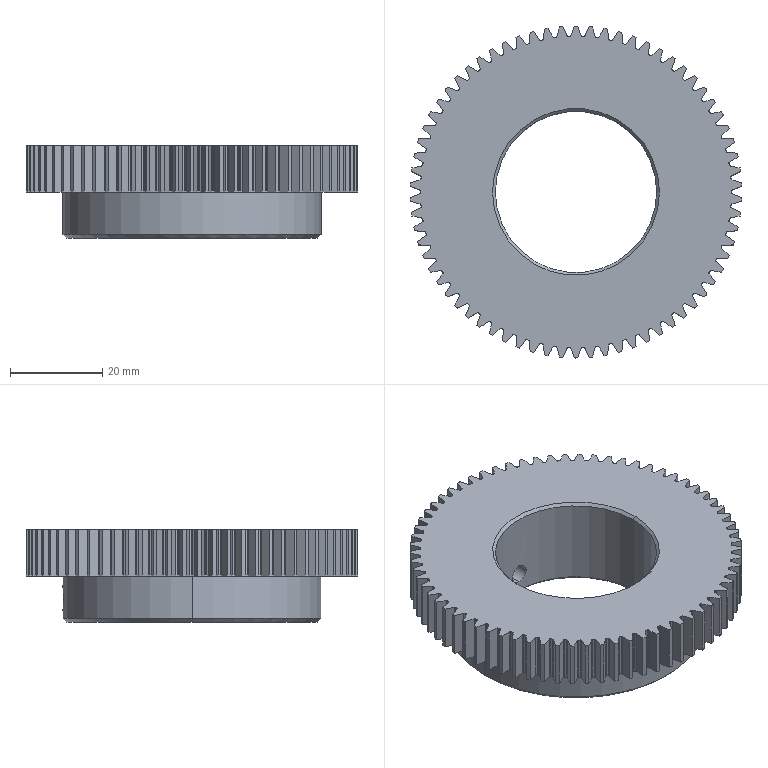Part | SolidWorks | features BaseBody 1 | 1 solid | 468 faces | box 71.959 x 72 x 20 mm | volume 43377 mm3 | cylinder 317 | plane 143 | cone 8 | commonest cylinder face diameters 0.5 x170 67.5 x71 72 x70 4.134 x2 35 x2 56 x2